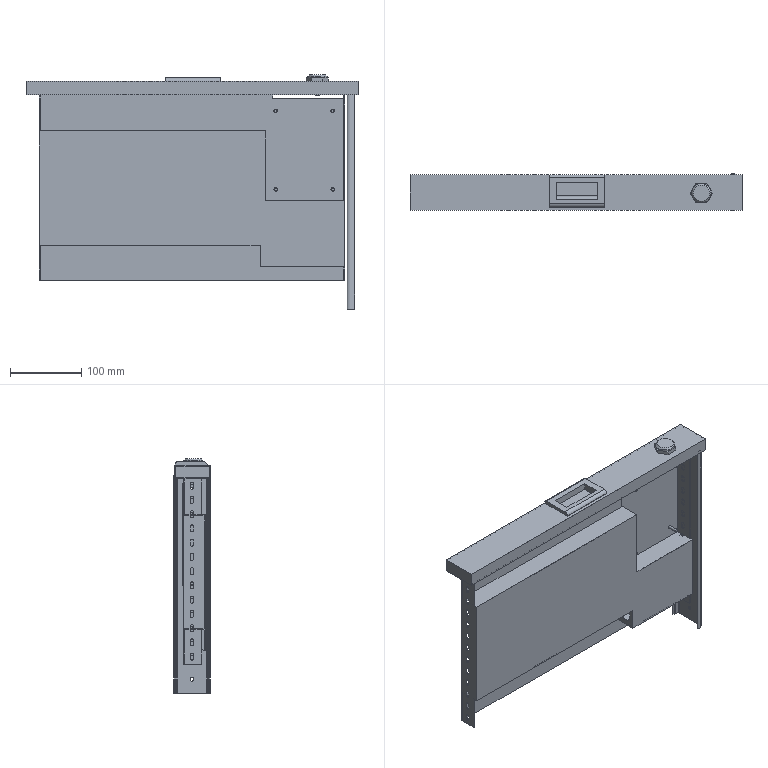Part | SolidWorks | 6 solids | 335 faces | box 466 x 51.75 x 328.5 mm | volume 398956 mm3 | plane 189 | cylinder 144 | cone 2 | commonest cylinder face diameters 5 x88 4.5 x18 4 x8 6 x5 18 x3 19 x3